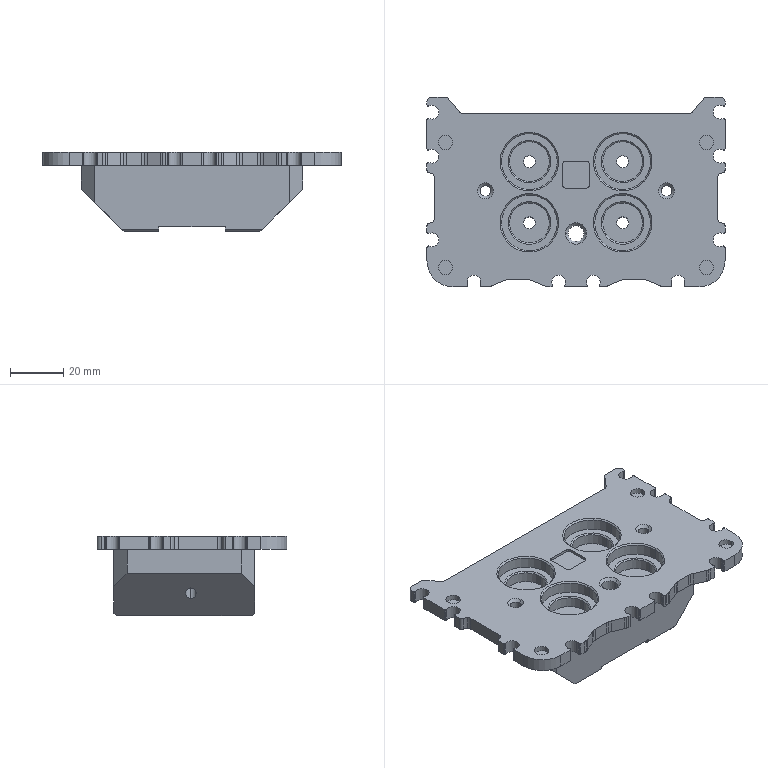Part | STEP file | ASND-0110-TPIM-023 | 1 solid | 263 faces | box 111.9 x 71.3 x 30 mm | volume 98030 mm3 | cylinder 157 | plane 76 | cone 30 | commonest cylinder face diameters 1 x40 4 x22 5.2 x21 10 x16 2 x12 4.5 x8